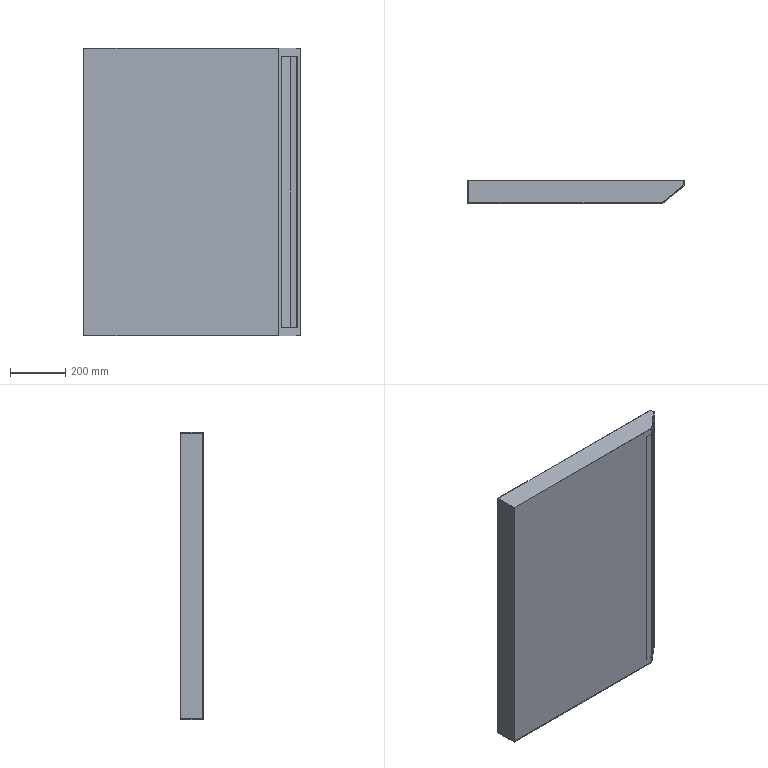Part | SolidWorks | features ICE 6, Extrusion 1, Shell 1 | 4 solids | 46 faces | box 782 x 83 x 1038 mm | volume 2557655 mm3 | plane 46
STEP:
#1=CARTESIAN_POINT('',(2.,2.,2.));
#2=VERTEX_POINT('',#1);
#3=CARTESIAN_POINT('',(703.425,2.,2.));
#4=VERTEX_POINT('',#3);
#5=CARTESIAN_POINT('',(0.,2.,2.));
#6=DIRECTION('',(1.,0.,0.));
#7=VECTOR('',#6,1000.);
#8=LINE('',#5,#7);
#9=EDGE_CURVE('',#2,#4,#8,.T.);
#10=ORIENTED_EDGE('',*,*,#9,.F.);
#11=CARTESIAN_POINT('',(2.,2.,1036.));
#12=VERTEX_POINT('',#11);
#13=CARTESIAN_POINT('',(2.,2.,1038.));
#14=DIRECTION('',(0.,0.,-1.));
#15=VECTOR('',#14,1000.);
#16=LINE('',#13,#15);
#17=EDGE_CURVE('',#12,#2,#16,.T.);
#18=ORIENTED_EDGE('',*,*,#17,.F.);
#19=CARTESIAN_POINT('',(703.425,2.,1036.));
#20=VERTEX_POINT('',#19);
#21=CARTESIAN_POINT('',(0.,2.,1036.));
#22=DIRECTION('',(1.,0.,0.));
#23=VECTOR('',#22,1000.);
#24=LINE('',#21,#23);
#25=EDGE_CURVE('',#12,#20,#24,.T.);
#26=ORIENTED_EDGE('',*,*,#25,.T.);
#27=CARTESIAN_POINT('',(703.425,2.,1038.));
#28=DIRECTION('',(0.,0.,-1.));
#29=VECTOR('',#28,1000.);
#30=LINE('',#27,#29);
#31=EDGE_CURVE('',#20,#4,#30,.T.);
#32=ORIENTED_EDGE('',*,*,#31,.T.);
#33=EDGE_LOOP('',(#10,#18,#26,#32));
#34=FACE_OUTER_BOUND('',#33,.T.);
#35=CARTESIAN_POINT('',(677.425,2.,1012.));
#36=VERTEX_POINT('',#35);
#37=CARTESIAN_POINT('',(679.425,2.,1012.));
#38=VERTEX_POINT('',#37);
#39=CARTESIAN_POINT('',(677.425,2.,1012.));
#40=DIRECTION('',(1.,0.,0.));
#41=VECTOR('',#40,1000.);
#42=LINE('',#39,#41);
#43=EDGE_CURVE('',#36,#38,#42,.T.);
#44=ORIENTED_EDGE('',*,*,#43,.F.);
#45=CARTESIAN_POINT('',(677.425,2.,26.));
#46=VERTEX_POINT('',#45);
#47=CARTESIAN_POINT('',(677.425,2.,26.));
#48=DIRECTION('',(0.,0.,1.));
#49=VECTOR('',#48,1000.);
#50=LINE('',#47,#49);
#51=EDGE_CURVE('',#46,#36,#50,.T.);
#52=ORIENTED_EDGE('',*,*,#51,.F.);
#53=CARTESIAN_POINT('',(679.425,2.,26.));
#54=VERTEX_POINT('',#53);
#55=CARTESIAN_POINT('',(677.425,2.,26.));
#56=DIRECTION('',(-1.,0.,0.));
#57=VECTOR('',#56,1000.);
#58=LINE('',#55,#57);
#59=EDGE_CURVE('',#54,#46,#58,.T.);
#60=ORIENTED_EDGE('',*,*,#59,.F.);
#61=CARTESIAN_POINT('',(679.425,2.,26.));
#62=DIRECTION('',(0.,0.,-1.));
#63=VECTOR('',#62,1000.);
#64=LINE('',#61,#63);
#65=EDGE_CURVE('',#38,#54,#64,.T.);
#66=ORIENTED_EDGE('',*,*,#65,.F.);
#67=EDGE_LOOP('',(#44,#52,#60,#66));
#68=FACE_BOUND('',#67,.T.);
#69=CARTESIAN_POINT('',(704.153,2.,1038.));
#70=DIRECTION('',(0.,1.,0.));
#71=DIRECTION('',(-1.,0.,0.));
#72=AXIS2_PLACEMENT_3D('',#69,#70,#71);
#73=PLANE('',#72);
#74=ADVANCED_FACE('',(#34,#68),#73,.T.);
#75=CARTESIAN_POINT('',(0.,0.,0.));
#76=VERTEX_POINT('',#75);
#77=CARTESIAN_POINT('',(704.153,0.,0.));
#78=VERTEX_POINT('',#77);
#79=CARTESIAN_POINT('',(704.153,0.,0.));
#80=DIRECTION('',(1.,0.,0.));
#81=VECTOR('',#80,1000.);
#82=LINE('',#79,#81);
#83=EDGE_CURVE('',#76,#78,#82,.T.);
#84=ORIENTED_EDGE('',*,*,#83,.T.);
#85=CARTESIAN_POINT('',(704.153,0.,1038.));
#86=VERTEX_POINT('',#85);
#87=CARTESIAN_POINT('',(704.153,0.,1038.));
#88=DIRECTION('',(0.,0.,-1.));
#89=VECTOR('',#88,1000.);
#90=LINE('',#87,#89);
#91=EDGE_CURVE('',#86,#78,#90,.T.);
#92=ORIENTED_EDGE('',*,*,#91,.F.);
#93=CARTESIAN_POINT('',(0.,0.,1038.));
#94=VERTEX_POINT('',#93);
#95=CARTESIAN_POINT('',(704.153,0.,1038.));
#96=DIRECTION('',(1.,0.,0.));
#97=VECTOR('',#96,1000.);
#98=LINE('',#95,#97);
#99=EDGE_CURVE('',#94,#86,#98,.T.);
#100=ORIENTED_EDGE('',*,*,#99,.F.);
#101=CARTESIAN_POINT('',(0.,0.,1038.));
#102=DIRECTION('',(0.,0.,-1.));
#103=VECTOR('',#102,1000.);
#104=LINE('',#101,#103);
#105=EDGE_CURVE('',#94,#76,#104,.T.);
#106=ORIENTED_EDGE('',*,*,#105,.T.);
#107=EDGE_LOOP('',(#84,#92,#100,#106));
#108=FACE_OUTER_BOUND('',#107,.T.);
#109=CARTESIAN_POINT('',(704.153,0.,1038.));
#110=DIRECTION('',(0.,1.,0.));
#111=DIRECTION('',(-1.,0.,0.));
#112=AXIS2_PLACEMENT_3D('',#109,#110,#111);
#113=PLANE('',#112);
#114=ADVANCED_FACE('',(#108),#113,.F.);
#115=CARTESIAN_POINT('',(714.35,8.556,28.));
#116=VERTEX_POINT('',#115);
#117=CARTESIAN_POINT('',(771.803,56.765,28.));
#118=VERTEX_POINT('',#117);
#119=CARTESIAN_POINT('',(714.35,8.556,28.));
#120=DIRECTION('',(0.766,0.6428,0.));
#121=VECTOR('',#120,1000.);
#122=LINE('',#119,#121);
#123=EDGE_CURVE('',#116,#118,#122,.T.);
#124=ORIENTED_EDGE('',*,*,#123,.F.);
#125=CARTESIAN_POINT('',(714.35,8.556,1010.));
#126=VERTEX_POINT('',#125);
#127=CARTESIAN_POINT('',(714.35,8.556,1010.));
#128=DIRECTION('',(0.,0.,-1.));
#129=VECTOR('',#128,1000.);
#130=LINE('',#127,#129);
#131=EDGE_CURVE('',#126,#116,#130,.T.);
#132=ORIENTED_EDGE('',*,*,#131,.F.);
#133=CARTESIAN_POINT('',(771.803,56.765,1010.));
#134=VERTEX_POINT('',#133);
#135=CARTESIAN_POINT('',(714.35,8.556,1010.));
#136=DIRECTION('',(-0.766,-0.6428,0.));
#137=VECTOR('',#136,1000.);
#138=LINE('',#135,#137);
#139=EDGE_CURVE('',#134,#126,#138,.T.);
#140=ORIENTED_EDGE('',*,*,#139,.F.);
#141=CARTESIAN_POINT('',(771.803,56.765,1010.));
#142=DIRECTION('',(0.,0.,1.));
#143=VECTOR('',#142,1000.);
#144=LINE('',#141,#143);
#145=EDGE_CURVE('',#118,#134,#144,.T.);
#146=ORIENTED_EDGE('',*,*,#145,.F.);
#147=EDGE_LOOP('',(#124,#132,#140,#146));
#148=FACE_BOUND('',#147,.T.);
#149=CARTESIAN_POINT('',(782.,65.322,0.));
#150=VERTEX_POINT('',#149);
#151=CARTESIAN_POINT('',(784.,67.,0.));
#152=DIRECTION('',(0.766,0.6428,0.));
#153=VECTOR('',#152,1000.);
#154=LINE('',#151,#153);
#155=EDGE_CURVE('',#78,#150,#154,.T.);
#156=ORIENTED_EDGE('',*,*,#155,.T.);
#157=CARTESIAN_POINT('',(782.,65.322,1038.));
#158=VERTEX_POINT('',#157);
#159=CARTESIAN_POINT('',(782.,65.322,1038.));
#160=DIRECTION('',(0.,0.,1.));
#161=VECTOR('',#160,1000.);
#162=LINE('',#159,#161);
#163=EDGE_CURVE('',#150,#158,#162,.T.);
#164=ORIENTED_EDGE('',*,*,#163,.T.);
#165=CARTESIAN_POINT('',(784.,67.,1038.));
#166=DIRECTION('',(0.766,0.6428,0.));
#167=VECTOR('',#166,1000.);
#168=LINE('',#165,#167);
#169=EDGE_CURVE('',#86,#158,#168,.T.);
#170=ORIENTED_EDGE('',*,*,#169,.F.);
#171=ORIENTED_EDGE('',*,*,#91,.T.);
#172=EDGE_LOOP('',(#156,#164,#170,#171));
#173=FACE_OUTER_BOUND('',#172,.T.);
#174=CARTESIAN_POINT('',(784.,67.,1038.));
#175=DIRECTION('',(-0.6428,0.766,0.));
#176=DIRECTION('',(-0.766,-0.6428,0.));
#177=AXIS2_PLACEMENT_3D('',#174,#175,#176);
#178=PLANE('',#177);
#179=ADVANCED_FACE('',(#148,#173),#178,.F.);
#180=CARTESIAN_POINT('',(780.,83.,1036.));
#181=VERTEX_POINT('',#180);
#182=CARTESIAN_POINT('',(780.,83.,2.));
#183=VERTEX_POINT('',#182);
#184=CARTESIAN_POINT('',(780.,83.,1038.));
#185=DIRECTION('',(0.,0.,-1.));
#186=VECTOR('',#185,1000.);
#187=LINE('',#184,#186);
#188=EDGE_CURVE('',#181,#183,#187,.T.);
#189=ORIENTED_EDGE('',*,*,#188,.F.);
#190=CARTESIAN_POINT('',(2.,83.,1036.));
#191=VERTEX_POINT('',#190);
#192=CARTESIAN_POINT('',(0.,83.,1036.));
#193=DIRECTION('',(-1.,0.,0.));
#194=VECTOR('',#193,1000.);
#195=LINE('',#192,#194);
#196=EDGE_CURVE('',#181,#191,#195,.T.);
#197=ORIENTED_EDGE('',*,*,#196,.T.);
#198=CARTESIAN_POINT('',(2.,83.,2.));
#199=VERTEX_POINT('',#198);
#200=CARTESIAN_POINT('',(2.,83.,1038.));
#201=DIRECTION('',(0.,0.,-1.));
#202=VECTOR('',#201,1000.);
#203=LINE('',#200,#202);
#204=EDGE_CURVE('',#191,#199,#203,.T.);
#205=ORIENTED_EDGE('',*,*,#204,.T.);
#206=CARTESIAN_POINT('',(0.,83.,2.));
#207=DIRECTION('',(-1.,0.,0.));
#208=VECTOR('',#207,1000.);
#209=LINE('',#206,#208);
#210=EDGE_CURVE('',#183,#199,#209,.T.);
#211=ORIENTED_EDGE('',*,*,#210,.F.);
#212=EDGE_LOOP('',(#189,#197,#205,#211));
#213=FACE_BOUND('',#212,.T.);
#214=CARTESIAN_POINT('',(782.,83.,1038.));
#215=VERTEX_POINT('',#214);
#216=CARTESIAN_POINT('',(0.,83.,1038.));
#217=VERTEX_POINT('',#216);
#218=CARTESIAN_POINT('',(0.,83.,1038.));
#219=DIRECTION('',(-1.,0.,0.));
#220=VECTOR('',#219,1000.);
#221=LINE('',#218,#220);
#222=EDGE_CURVE('',#215,#217,#221,.T.);
#223=ORIENTED_EDGE('',*,*,#222,.F.);
#224=CARTESIAN_POINT('',(782.,83.,0.));
#225=VERTEX_POINT('',#224);
#226=CARTESIAN_POINT('',(782.,83.,1038.));
#227=DIRECTION('',(0.,0.,-1.));
#228=VECTOR('',#227,1000.);
#229=LINE('',#226,#228);
#230=EDGE_CURVE('',#215,#225,#229,.T.);
#231=ORIENTED_EDGE('',*,*,#230,.T.);
#232=CARTESIAN_POINT('',(0.,83.,0.));
#233=VERTEX_POINT('',#232);
#234=CARTESIAN_POINT('',(0.,83.,0.));
#235=DIRECTION('',(-1.,0.,0.));
#236=VECTOR('',#235,1000.);
#237=LINE('',#234,#236);
#238=EDGE_CURVE('',#225,#233,#237,.T.);
#239=ORIENTED_EDGE('',*,*,#238,.T.);
#240=CARTESIAN_POINT('',(0.,83.,1038.));
#241=DIRECTION('',(0.,0.,-1.));
#242=VECTOR('',#241,1000.);
#243=LINE('',#240,#242);
#244=EDGE_CURVE('',#217,#233,#243,.T.);
#245=ORIENTED_EDGE('',*,*,#244,.F.);
#246=EDGE_LOOP('',(#223,#231,#239,#245));
#247=FACE_OUTER_BOUND('',#246,.T.);
#248=CARTESIAN_POINT('',(0.,83.,1038.));
#249=DIRECTION('',(0.,-1.,0.));
#250=DIRECTION('',(0.,0.,-1.));
#251=AXIS2_PLACEMENT_3D('',#248,#249,#250);
#252=PLANE('',#251);
#253=ADVANCED_FACE('',(#213,#247),#252,.F.);
#254=CARTESIAN_POINT('',(0.,0.,0.));
#255=DIRECTION('',(0.,-1.,0.));
#256=VECTOR('',#255,1000.);
#257=LINE('',#254,#256);
#258=EDGE_CURVE('',#233,#76,#257,.T.);
#259=ORIENTED_EDGE('',*,*,#258,.T.);
#260=ORIENTED_EDGE('',*,*,#105,.F.);
#261=CARTESIAN_POINT('',(0.,0.,1038.));
#262=DIRECTION('',(0.,-1.,0.));
#263=VECTOR('',#262,1000.);
#264=LINE('',#261,#263);
#265=EDGE_CURVE('',#217,#94,#264,.T.);
#266=ORIENTED_EDGE('',*,*,#265,.F.);
#267=ORIENTED_EDGE('',*,*,#244,.T.);
#268=EDGE_LOOP('',(#259,#260,#266,#267));
#269=FACE_OUTER_BOUND('',#268,.T.);
#270=CARTESIAN_POINT('',(0.,0.,1038.));
#271=DIRECTION('',(1.,0.,0.));
#272=DIRECTION('',(0.,0.,-1.));
#273=AXIS2_PLACEMENT_3D('',#270,#271,#272);
#274=PLANE('',#273);
#275=ADVANCED_FACE('',(#269),#274,.F.);
#276=ORIENTED_EDGE('',*,*,#169,.T.);
#277=CARTESIAN_POINT('',(782.,134.153,1038.));
#278=DIRECTION('',(0.,-1.,0.));
#279=VECTOR('',#278,1000.);
#280=LINE('',#277,#279);
#281=EDGE_CURVE('',#215,#158,#280,.T.);
#282=ORIENTED_EDGE('',*,*,#281,.F.);
#283=ORIENTED_EDGE('',*,*,#222,.T.);
#284=ORIENTED_EDGE('',*,*,#265,.T.);
#285=ORIENTED_EDGE('',*,*,#99,.T.);
#286=EDGE_LOOP('',(#276,#282,#283,#284,#285));
#287=FACE_OUTER_BOUND('',#286,.T.);
#288=CARTESIAN_POINT('',(0.,0.,1038.));
#289=DIRECTION('',(0.,0.,-1.));
#290=DIRECTION('',(-1.,0.,0.));
#291=AXIS2_PLACEMENT_3D('',#288,#289,#290);
#292=PLANE('',#291);
#293=ADVANCED_FACE('',(#287),#292,.F.);
#294=CARTESIAN_POINT('',(782.,0.,0.));
#295=DIRECTION('',(0.,1.,0.));
#296=VECTOR('',#295,1000.);
#297=LINE('',#294,#296);
#298=EDGE_CURVE('',#150,#225,#297,.T.);
#299=ORIENTED_EDGE('',*,*,#298,.F.);
#300=ORIENTED_EDGE('',*,*,#155,.F.);
#301=ORIENTED_EDGE('',*,*,#83,.F.);
#302=ORIENTED_EDGE('',*,*,#258,.F.);
#303=ORIENTED_EDGE('',*,*,#238,.F.);
#304=EDGE_LOOP('',(#299,#300,#301,#302,#303));
#305=FACE_OUTER_BOUND('',#304,.T.);
#306=CARTESIAN_POINT('',(0.,0.,0.));
#307=DIRECTION('',(0.,0.,-1.));
#308=DIRECTION('',(-1.,0.,0.));
#309=AXIS2_PLACEMENT_3D('',#306,#307,#308);
#310=PLANE('',#309);
#311=ADVANCED_FACE('',(#305),#310,.T.);
#312=ORIENTED_EDGE('',*,*,#298,.T.);
#313=ORIENTED_EDGE('',*,*,#230,.F.);
#314=ORIENTED_EDGE('',*,*,#281,.T.);
#315=ORIENTED_EDGE('',*,*,#163,.F.);
#316=EDGE_LOOP('',(#312,#313,#314,#315));
#317=FACE_OUTER_BOUND('',#316,.T.);
#318=CARTESIAN_POINT('',(782.,134.153,-153.));
#319=DIRECTION('',(-1.,0.,0.));
#320=DIRECTION('',(0.,0.,1.));
#321=AXIS2_PLACEMENT_3D('',#318,#319,#320);
#322=PLANE('',#321);
#323=ADVANCED_FACE('',(#317),#322,.F.);
#324=CARTESIAN_POINT('',(713.064,10.088,28.));
#325=VERTEX_POINT('',#324);
#326=CARTESIAN_POINT('',(713.064,10.088,1010.));
#327=VERTEX_POINT('',#326);
#328=CARTESIAN_POINT('',(713.064,10.088,1038.));
#329=DIRECTION('',(0.,0.,1.));
#330=VECTOR('',#329,1000.);
#331=LINE('',#328,#330);
#332=EDGE_CURVE('',#325,#327,#331,.T.);
#333=ORIENTED_EDGE('',*,*,#332,.F.);
#334=CARTESIAN_POINT('',(770.517,58.298,28.));
#335=VERTEX_POINT('',#334);
#336=CARTESIAN_POINT('',(782.714,68.532,28.));
#337=DIRECTION('',(-0.766,-0.6428,0.));
#338=VECTOR('',#337,1000.);
#339=LINE('',#336,#338);
#340=EDGE_CURVE('',#335,#325,#339,.T.);
#341=ORIENTED_EDGE('',*,*,#340,.F.);
#342=CARTESIAN_POINT('',(770.517,58.298,1010.));
#343=VERTEX_POINT('',#342);
#344=CARTESIAN_POINT('',(770.517,58.298,1038.));
#345=DIRECTION('',(0.,0.,-1.));
#346=VECTOR('',#345,1000.);
#347=LINE('',#344,#346);
#348=EDGE_CURVE('',#343,#335,#347,.T.);
#349=ORIENTED_EDGE('',*,*,#348,.F.);
#350=CARTESIAN_POINT('',(782.714,68.532,1010.));
#351=DIRECTION('',(0.766,0.6428,0.));
#352=VECTOR('',#351,1000.);
#353=LINE('',#350,#352);
#354=EDGE_CURVE('',#327,#343,#353,.T.);
#355=ORIENTED_EDGE('',*,*,#354,.F.);
#356=EDGE_LOOP('',(#333,#341,#349,#355));
#357=FACE_BOUND('',#356,.T.);
#358=CARTESIAN_POINT('',(780.,66.254,2.));
#359=VERTEX_POINT('',#358);
#360=CARTESIAN_POINT('',(289.653,-345.195,2.));
#361=DIRECTION('',(0.766,0.6428,0.));
#362=VECTOR('',#361,1000.);
#363=LINE('',#360,#362);
#364=EDGE_CURVE('',#4,#359,#363,.T.);
#365=ORIENTED_EDGE('',*,*,#364,.F.);
#366=ORIENTED_EDGE('',*,*,#31,.F.);
#367=CARTESIAN_POINT('',(780.,66.254,1036.));
#368=VERTEX_POINT('',#367);
#369=CARTESIAN_POINT('',(289.653,-345.195,1036.));
#370=DIRECTION('',(0.766,0.6428,0.));
#371=VECTOR('',#370,1000.);
#372=LINE('',#369,#371);
#373=EDGE_CURVE('',#20,#368,#372,.T.);
#374=ORIENTED_EDGE('',*,*,#373,.T.);
#375=CARTESIAN_POINT('',(780.,66.254,1038.));
#376=DIRECTION('',(0.,0.,1.));
#377=VECTOR('',#376,1000.);
#378=LINE('',#375,#377);
#379=EDGE_CURVE('',#359,#368,#378,.T.);
#380=ORIENTED_EDGE('',*,*,#379,.F.);
#381=EDGE_LOOP('',(#365,#366,#374,#380));
#382=FACE_OUTER_BOUND('',#381,.T.);
#383=CARTESIAN_POINT('',(782.714,68.532,1038.));
#384=DIRECTION('',(-0.6428,0.766,0.));
#385=DIRECTION('',(-0.766,-0.6428,0.));
#386=AXIS2_PLACEMENT_3D('',#383,#384,#385);
#387=PLANE('',#386);
#388=ADVANCED_FACE('',(#357,#382),#387,.T.);
#389=CARTESIAN_POINT('',(2.,0.,2.));
#390=DIRECTION('',(0.,-1.,0.));
#391=VECTOR('',#390,1000.);
#392=LINE('',#389,#391);
#393=EDGE_CURVE('',#199,#2,#392,.T.);
#394=ORIENTED_EDGE('',*,*,#393,.F.);
#395=ORIENTED_EDGE('',*,*,#204,.F.);
#396=CARTESIAN_POINT('',(2.,0.,1036.));
#397=DIRECTION('',(0.,-1.,0.));
#398=VECTOR('',#397,1000.);
#399=LINE('',#396,#398);
#400=EDGE_CURVE('',#191,#12,#399,.T.);
#401=ORIENTED_EDGE('',*,*,#400,.T.);
#402=ORIENTED_EDGE('',*,*,#17,.T.);
#403=EDGE_LOOP('',(#394,#395,#401,#402));
#404=FACE_OUTER_BOUND('',#403,.T.);
#405=CARTESIAN_POINT('',(2.,0.,1038.));
#406=DIRECTION('',(1.,0.,0.));
#407=DIRECTION('',(0.,0.,-1.));
#408=AXIS2_PLACEMENT_3D('',#405,#406,#407);
#409=PLANE('',#408);
#410=ADVANCED_FACE('',(#404),#409,.T.);
#411=ORIENTED_EDGE('',*,*,#373,.F.);
#412=ORIENTED_EDGE('',*,*,#25,.F.);
#413=ORIENTED_EDGE('',*,*,#400,.F.);
#414=ORIENTED_EDGE('',*,*,#196,.F.);
#415=CARTESIAN_POINT('',(780.,134.153,1036.));
#416=DIRECTION('',(0.,-1.,0.));
#417=VECTOR('',#416,1000.);
#418=LINE('',#415,#417);
#419=EDGE_CURVE('',#181,#368,#418,.T.);
#420=ORIENTED_EDGE('',*,*,#419,.T.);
#421=EDGE_LOOP('',(#411,#412,#413,#414,#420));
#422=FACE_OUTER_BOUND('',#421,.T.);
#423=CARTESIAN_POINT('',(0.,0.,1036.));
#424=DIRECTION('',(0.,0.,-1.));
#425=DIRECTION('',(-1.,0.,0.));
#426=AXIS2_PLACEMENT_3D('',#423,#424,#425);
#427=PLANE('',#426);
#428=ADVANCED_FACE('',(#422),#427,.T.);
#429=CARTESIAN_POINT('',(780.,0.,2.));
#430=DIRECTION('',(0.,1.,0.));
#431=VECTOR('',#430,1000.);
#432=LINE('',#429,#431);
#433=EDGE_CURVE('',#359,#183,#432,.T.);
#434=ORIENTED_EDGE('',*,*,#433,.T.);
#435=ORIENTED_EDGE('',*,*,#210,.T.);
#436=ORIENTED_EDGE('',*,*,#393,.T.);
#437=ORIENTED_EDGE('',*,*,#9,.T.);
#438=ORIENTED_EDGE('',*,*,#364,.T.);
#439=EDGE_LOOP('',(#434,#435,#436,#437,#438));
#440=FACE_OUTER_BOUND('',#439,.T.);
#441=CARTESIAN_POINT('',(0.,0.,2.));
#442=DIRECTION('',(0.,0.,-1.));
#443=DIRECTION('',(-1.,0.,0.));
#444=AXIS2_PLACEMENT_3D('',#441,#442,#443);
#445=PLANE('',#444);
#446=ADVANCED_FACE('',(#440),#445,.F.);
#447=ORIENTED_EDGE('',*,*,#433,.F.);
#448=ORIENTED_EDGE('',*,*,#379,.T.);
#449=ORIENTED_EDGE('',*,*,#419,.F.);
#450=ORIENTED_EDGE('',*,*,#188,.T.);
#451=EDGE_LOOP('',(#447,#448,#449,#450));
#452=FACE_OUTER_BOUND('',#451,.T.);
#453=CARTESIAN_POINT('',(780.,134.153,-153.));
#454=DIRECTION('',(-1.,0.,0.));
#455=DIRECTION('',(0.,0.,1.));
#456=AXIS2_PLACEMENT_3D('',#453,#454,#455);
#457=PLANE('',#456);
#458=ADVANCED_FACE('',(#452),#457,.T.);
#459=ORIENTED_EDGE('',*,*,#332,.T.);
#460=CARTESIAN_POINT('',(293.966,509.549,1010.));
#461=DIRECTION('',(0.6428,-0.766,0.));
#462=VECTOR('',#461,1000.);
#463=LINE('',#460,#462);
#464=EDGE_CURVE('',#327,#126,#463,.T.);
#465=ORIENTED_EDGE('',*,*,#464,.T.);
#466=ORIENTED_EDGE('',*,*,#131,.T.);
#467=CARTESIAN_POINT('',(293.966,509.549,28.));
#468=DIRECTION('',(0.6428,-0.766,0.));
#469=VECTOR('',#468,1000.);
#470=LINE('',#467,#469);
#471=EDGE_CURVE('',#325,#116,#470,.T.);
#472=ORIENTED_EDGE('',*,*,#471,.F.);
#473=EDGE_LOOP('',(#459,#465,#466,#472));
#474=FACE_OUTER_BOUND('',#473,.T.);
#475=CARTESIAN_POINT('',(293.966,509.549,1010.));
#476=DIRECTION('',(-0.766,-0.6428,0.));
#477=DIRECTION('',(0.6428,-0.766,0.));
#478=AXIS2_PLACEMENT_3D('',#475,#476,#477);
#479=PLANE('',#478);
#480=ADVANCED_FACE('',(#474),#479,.F.);
#481=ORIENTED_EDGE('',*,*,#354,.T.);
#482=CARTESIAN_POINT('',(351.42,557.759,1010.));
#483=DIRECTION('',(0.6428,-0.766,0.));
#484=VECTOR('',#483,1000.);
#485=LINE('',#482,#484);
#486=EDGE_CURVE('',#343,#134,#485,.T.);
#487=ORIENTED_EDGE('',*,*,#486,.T.);
#488=ORIENTED_EDGE('',*,*,#139,.T.);
#489=ORIENTED_EDGE('',*,*,#464,.F.);
#490=EDGE_LOOP('',(#481,#487,#488,#489));
#491=FACE_OUTER_BOUND('',#490,.T.);
#492=CARTESIAN_POINT('',(293.966,509.549,1010.));
#493=DIRECTION('',(0.,0.,1.));
#494=DIRECTION('',(1.,0.,0.));
#495=AXIS2_PLACEMENT_3D('',#492,#493,#494);
#496=PLANE('',#495);
#497=ADVANCED_FACE('',(#491),#496,.F.);
#498=ORIENTED_EDGE('',*,*,#348,.T.);
#499=CARTESIAN_POINT('',(351.42,557.759,28.));
#500=DIRECTION('',(0.6428,-0.766,0.));
#501=VECTOR('',#500,1000.);
#502=LINE('',#499,#501);
#503=EDGE_CURVE('',#335,#118,#502,.T.);
#504=ORIENTED_EDGE('',*,*,#503,.T.);
#505=ORIENTED_EDGE('',*,*,#145,.T.);
#506=ORIENTED_EDGE('',*,*,#486,.F.);
#507=EDGE_LOOP('',(#498,#504,#505,#506));
#508=FACE_OUTER_BOUND('',#507,.T.);
#509=CARTESIAN_POINT('',(351.42,557.759,1010.));
#510=DIRECTION('',(0.766,0.6428,0.));
#511=DIRECTION('',(-0.6428,0.766,0.));
#512=AXIS2_PLACEMENT_3D('',#509,#510,#511);
#513=PLANE('',#512);
#514=ADVANCED_FACE('',(#508),#513,.F.);
#515=ORIENTED_EDGE('',*,*,#340,.T.);
#516=ORIENTED_EDGE('',*,*,#471,.T.);
#517=ORIENTED_EDGE('',*,*,#123,.T.);
#518=ORIENTED_EDGE('',*,*,#503,.F.);
#519=EDGE_LOOP('',(#515,#516,#517,#518));
#520=FACE_OUTER_BOUND('',#519,.T.);
#521=CARTESIAN_POINT('',(293.966,509.549,28.));
#522=DIRECTION('',(0.,0.,-1.));
#523=DIRECTION('',(-1.,0.,0.));
#524=AXIS2_PLACEMENT_3D('',#521,#522,#523);
#525=PLANE('',#524);
#526=ADVANCED_FACE('',(#520),#525,.F.);
#527=ORIENTED_EDGE('',*,*,#51,.T.);
#528=CARTESIAN_POINT('',(677.425,62.,1012.));
#529=VERTEX_POINT('',#528);
#530=CARTESIAN_POINT('',(677.425,62.,1012.));
#531=DIRECTION('',(0.,-1.,0.));
#532=VECTOR('',#531,1000.);
#533=LINE('',#530,#532);
#534=EDGE_CURVE('',#529,#36,#533,.T.);
#535=ORIENTED_EDGE('',*,*,#534,.F.);
#536=CARTESIAN_POINT('',(677.425,62.,26.));
#537=VERTEX_POINT('',#536);
#538=CARTESIAN_POINT('',(677.425,62.,26.));
#539=DIRECTION('',(0.,0.,1.));
#540=VECTOR('',#539,1000.);
#541=LINE('',#538,#540);
#542=EDGE_CURVE('',#537,#529,#541,.T.);
#543=ORIENTED_EDGE('',*,*,#542,.F.);
#544=CARTESIAN_POINT('',(677.425,62.,26.));
#545=DIRECTION('',(0.,-1.,0.));
#546=VECTOR('',#545,1000.);
#547=LINE('',#544,#546);
#548=EDGE_CURVE('',#537,#46,#547,.T.);
#549=ORIENTED_EDGE('',*,*,#548,.T.);
#550=EDGE_LOOP('',(#527,#535,#543,#549));
#551=FACE_OUTER_BOUND('',#550,.T.);
#552=CARTESIAN_POINT('',(677.425,62.,26.));
#553=DIRECTION('',(1.,0.,0.));
#554=DIRECTION('',(0.,1.,0.));
#555=AXIS2_PLACEMENT_3D('',#552,#553,#554);
#556=PLANE('',#555);
#557=ADVANCED_FACE('',(#551),#556,.F.);
#558=ORIENTED_EDGE('',*,*,#43,.T.);
#559=CARTESIAN_POINT('',(679.425,62.,1012.));
#560=VERTEX_POINT('',#559);
#561=CARTESIAN_POINT('',(679.425,62.,1012.));
#562=DIRECTION('',(0.,-1.,0.));
#563=VECTOR('',#562,1000.);
#564=LINE('',#561,#563);
#565=EDGE_CURVE('',#560,#38,#564,.T.);
#566=ORIENTED_EDGE('',*,*,#565,.F.);
#567=CARTESIAN_POINT('',(677.425,62.,1012.));
#568=DIRECTION('',(1.,0.,0.));
#569=VECTOR('',#568,1000.);
#570=LINE('',#567,#569);
#571=EDGE_CURVE('',#529,#560,#570,.T.);
#572=ORIENTED_EDGE('',*,*,#571,.F.);
#573=ORIENTED_EDGE('',*,*,#534,.T.);
#574=EDGE_LOOP('',(#558,#566,#572,#573));
#575=FACE_OUTER_BOUND('',#574,.T.);
#576=CARTESIAN_POINT('',(677.425,62.,1012.));
#577=DIRECTION('',(0.,0.,-1.));
#578=DIRECTION('',(-1.,0.,0.));
#579=AXIS2_PLACEMENT_3D('',#576,#577,#578);
#580=PLANE('',#579);
#581=ADVANCED_FACE('',(#575),#580,.F.);
#582=ORIENTED_EDGE('',*,*,#65,.T.);
#583=CARTESIAN_POINT('',(679.425,62.,26.));
#584=VERTEX_POINT('',#583);
#585=CARTESIAN_POINT('',(679.425,62.,26.));
#586=DIRECTION('',(0.,-1.,0.));
#587=VECTOR('',#586,1000.);
#588=LINE('',#585,#587);
#589=EDGE_CURVE('',#584,#54,#588,.T.);
#590=ORIENTED_EDGE('',*,*,#589,.F.);
#591=CARTESIAN_POINT('',(679.425,62.,26.));
#592=DIRECTION('',(0.,0.,-1.));
#593=VECTOR('',#592,1000.);
#594=LINE('',#591,#593);
#595=EDGE_CURVE('',#560,#584,#594,.T.);
#596=ORIENTED_EDGE('',*,*,#595,.F.);
#597=ORIENTED_EDGE('',*,*,#565,.T.);
#598=EDGE_LOOP('',(#582,#590,#596,#597));
#599=FACE_OUTER_BOUND('',#598,.T.);
#600=CARTESIAN_POINT('',(679.425,62.,26.));
#601=DIRECTION('',(-1.,0.,0.));
#602=DIRECTION('',(0.,0.,1.));
#603=AXIS2_PLACEMENT_3D('',#600,#601,#602);
#604=PLANE('',#603);
#605=ADVANCED_FACE('',(#599),#604,.F.);
#606=ORIENTED_EDGE('',*,*,#59,.T.);
#607=ORIENTED_EDGE('',*,*,#548,.F.);
#608=CARTESIAN_POINT('',(677.425,62.,26.));
#609=DIRECTION('',(-1.,0.,0.));
#610=VECTOR('',#609,1000.);
#611=LINE('',#608,#610);
#612=EDGE_CURVE('',#584,#537,#611,.T.);
#613=ORIENTED_EDGE('',*,*,#612,.F.);
#614=ORIENTED_EDGE('',*,*,#589,.T.);
#615=EDGE_LOOP('',(#606,#607,#613,#614));
#616=FACE_OUTER_BOUND('',#615,.T.);
#617=CARTESIAN_POINT('',(677.425,62.,26.));
#618=DIRECTION('',(0.,0.,1.));
#619=DIRECTION('',(1.,0.,0.));
#620=AXIS2_PLACEMENT_3D('',#617,#618,#619);
#621=PLANE('',#620);
#622=ADVANCED_FACE('',(#616),#621,.F.);
#623=ORIENTED_EDGE('',*,*,#542,.T.);
#624=ORIENTED_EDGE('',*,*,#571,.T.);
#625=ORIENTED_EDGE('',*,*,#595,.T.);
#626=ORIENTED_EDGE('',*,*,#612,.T.);
#627=EDGE_LOOP('',(#623,#624,#625,#626));
#628=FACE_OUTER_BOUND('',#627,.T.);
#629=CARTESIAN_POINT('',(677.425,62.,1012.));
#630=DIRECTION('',(0.,1.,0.));
#631=DIRECTION('',(0.,0.,1.));
#632=AXIS2_PLACEMENT_3D('',#629,#630,#631);
#633=PLANE('',#632);
#634=ADVANCED_FACE('',(#628),#633,.T.);
#635=CLOSED_SHELL('',(#74,#114,#179,#253,#275,#293,#311,#323,#388,#410,#428,#446,#458,#480,#497,#514,#526,#557,#581,#605,#622,#634));
#636=MANIFOLD_SOLID_BREP('',#635);
#637=CARTESIAN_POINT('',(679.425,2.,26.));
#638=VERTEX_POINT('',#637);
#639=CARTESIAN_POINT('',(679.425,2.,1012.));
#640=VERTEX_POINT('',#639);
#641=CARTESIAN_POINT('',(679.425,2.,26.));
#642=DIRECTION('',(0.,0.,1.));
#643=VECTOR('',#642,1000.);
#644=LINE('',#641,#643);
#645=EDGE_CURVE('',#638,#640,#644,.T.);
#646=ORIENTED_EDGE('',*,*,#645,.T.);
#647=CARTESIAN_POINT('',(679.425,62.,1012.));
#648=VERTEX_POINT('',#647);
#649=CARTESIAN_POINT('',(679.425,62.,1012.));
#650=DIRECTION('',(0.,-1.,0.));
#651=VECTOR('',#650,1000.);
#652=LINE('',#649,#651);
#653=EDGE_CURVE('',#648,#640,#652,.T.);
#654=ORIENTED_EDGE('',*,*,#653,.F.);
#655=CARTESIAN_POINT('',(679.425,62.,26.));
#656=VERTEX_POINT('',#655);
#657=CARTESIAN_POINT('',(679.425,62.,26.));
#658=DIRECTION('',(0.,0.,1.));
#659=VECTOR('',#658,1000.);
#660=LINE('',#657,#659);
#661=EDGE_CURVE('',#656,#648,#660,.T.);
#662=ORIENTED_EDGE('',*,*,#661,.F.);
#663=CARTESIAN_POINT('',(679.425,62.,26.));
#664=DIRECTION('',(0.,-1.,0.));
#665=VECTOR('',#664,1000.);
#666=LINE('',#663,#665);
#667=EDGE_CURVE('',#656,#638,#666,.T.);
#668=ORIENTED_EDGE('',*,*,#667,.T.);
#669=EDGE_LOOP('',(#646,#654,#662,#668));
#670=FACE_OUTER_BOUND('',#669,.T.);
#671=CARTESIAN_POINT('',(679.425,62.,26.));
#672=DIRECTION('',(-1.,0.,0.));
#673=DIRECTION('',(0.,0.,1.));
#674=AXIS2_PLACEMENT_3D('',#671,#672,#673);
#675=PLANE('',#674);
#676=ADVANCED_FACE('',(#670),#675,.T.);
#677=ORIENTED_EDGE('',*,*,#661,.T.);
#678=CARTESIAN_POINT('',(774.93,62.,1012.));
#679=VERTEX_POINT('',#678);
#680=CARTESIAN_POINT('',(679.425,62.,1012.));
#681=DIRECTION('',(-1.,0.,0.));
#682=VECTOR('',#681,1000.);
#683=LINE('',#680,#682);
#684=EDGE_CURVE('',#679,#648,#683,.T.);
#685=ORIENTED_EDGE('',*,*,#684,.F.);
#686=CARTESIAN_POINT('',(774.93,62.,26.));
#687=VERTEX_POINT('',#686);
#688=CARTESIAN_POINT('',(774.93,62.,26.));
#689=DIRECTION('',(0.,0.,1.));
#690=VECTOR('',#689,1000.);
#691=LINE('',#688,#690);
#692=EDGE_CURVE('',#687,#679,#691,.T.);
#693=ORIENTED_EDGE('',*,*,#692,.F.);
#694=CARTESIAN_POINT('',(679.425,62.,26.));
#695=DIRECTION('',(-1.,0.,0.));
#696=VECTOR('',#695,1000.);
#697=LINE('',#694,#696);
#698=EDGE_CURVE('',#687,#656,#697,.T.);
#699=ORIENTED_EDGE('',*,*,#698,.T.);
#700=EDGE_LOOP('',(#677,#685,#693,#699));
#701=FACE_OUTER_BOUND('',#700,.T.);
#702=CARTESIAN_POINT('',(679.425,62.,26.));
#703=DIRECTION('',(0.,1.,0.));
#704=DIRECTION('',(-1.,0.,0.));
#705=AXIS2_PLACEMENT_3D('',#702,#703,#704);
#706=PLANE('',#705);
#707=ADVANCED_FACE('',(#701),#706,.T.);
#708=ORIENTED_EDGE('',*,*,#692,.T.);
#709=CARTESIAN_POINT('',(772.546,60.,1012.));
#710=VERTEX_POINT('',#709);
#711=CARTESIAN_POINT('',(774.93,62.,1012.));
#712=DIRECTION('',(0.766,0.6428,0.));
#713=VECTOR('',#712,1000.);
#714=LINE('',#711,#713);
#715=EDGE_CURVE('',#710,#679,#714,.T.);
#716=ORIENTED_EDGE('',*,*,#715,.F.);
#717=CARTESIAN_POINT('',(772.546,60.,26.));
#718=VERTEX_POINT('',#717);
#719=CARTESIAN_POINT('',(772.546,60.,26.));
#720=DIRECTION('',(0.,0.,1.));
#721=VECTOR('',#720,1000.);
#722=LINE('',#719,#721);
#723=EDGE_CURVE('',#718,#710,#722,.T.);
#724=ORIENTED_EDGE('',*,*,#723,.F.);
#725=CARTESIAN_POINT('',(774.93,62.,26.));
#726=DIRECTION('',(0.766,0.6428,0.));
#727=VECTOR('',#726,1000.);
#728=LINE('',#725,#727);
#729=EDGE_CURVE('',#718,#687,#728,.T.);
#730=ORIENTED_EDGE('',*,*,#729,.T.);
#731=EDGE_LOOP('',(#708,#716,#724,#730));
#732=FACE_OUTER_BOUND('',#731,.T.);
#733=CARTESIAN_POINT('',(774.93,62.,26.));
#734=DIRECTION('',(0.6428,-0.766,0.));
#735=DIRECTION('',(0.766,0.6428,0.));
#736=AXIS2_PLACEMENT_3D('',#733,#734,#735);
#737=PLANE('',#736);
#738=ADVANCED_FACE('',(#732),#737,.T.);
#739=ORIENTED_EDGE('',*,*,#723,.T.);
#740=CARTESIAN_POINT('',(681.425,60.,1012.));
#741=VERTEX_POINT('',#740);
#742=CARTESIAN_POINT('',(681.425,60.,1012.));
#743=DIRECTION('',(1.,0.,0.));
#744=VECTOR('',#743,1000.);
#745=LINE('',#742,#744);
#746=EDGE_CURVE('',#741,#710,#745,.T.);
#747=ORIENTED_EDGE('',*,*,#746,.F.);
#748=CARTESIAN_POINT('',(681.425,60.,26.));
#749=VERTEX_POINT('',#748);
#750=CARTESIAN_POINT('',(681.425,60.,26.));
#751=DIRECTION('',(0.,0.,1.));
#752=VECTOR('',#751,1000.);
#753=LINE('',#750,#752);
#754=EDGE_CURVE('',#749,#741,#753,.T.);
#755=ORIENTED_EDGE('',*,*,#754,.F.);
#756=CARTESIAN_POINT('',(681.425,60.,26.));
#757=DIRECTION('',(1.,0.,0.));
#758=VECTOR('',#757,1000.);
#759=LINE('',#756,#758);
#760=EDGE_CURVE('',#749,#718,#759,.T.);
#761=ORIENTED_EDGE('',*,*,#760,.T.);
#762=EDGE_LOOP('',(#739,#747,#755,#761));
#763=FACE_OUTER_BOUND('',#762,.T.);
#764=CARTESIAN_POINT('',(681.425,60.,26.));
#765=DIRECTION('',(0.,-1.,0.));
#766=DIRECTION('',(0.,0.,-1.));
#767=AXIS2_PLACEMENT_3D('',#764,#765,#766);
#768=PLANE('',#767);
#769=ADVANCED_FACE('',(#763),#768,.T.);
#770=ORIENTED_EDGE('',*,*,#754,.T.);
#771=CARTESIAN_POINT('',(681.425,4.,1012.));
#772=VERTEX_POINT('',#771);
#773=CARTESIAN_POINT('',(681.425,60.,1012.));
#774=DIRECTION('',(0.,1.,0.));
#775=VECTOR('',#774,1000.);
#776=LINE('',#773,#775);
#777=EDGE_CURVE('',#772,#741,#776,.T.);
#778=ORIENTED_EDGE('',*,*,#777,.F.);
#779=CARTESIAN_POINT('',(681.425,4.,26.));
#780=VERTEX_POINT('',#779);
#781=CARTESIAN_POINT('',(681.425,4.,26.));
#782=DIRECTION('',(0.,0.,1.));
#783=VECTOR('',#782,1000.);
#784=LINE('',#781,#783);
#785=EDGE_CURVE('',#780,#772,#784,.T.);
#786=ORIENTED_EDGE('',*,*,#785,.F.);
#787=CARTESIAN_POINT('',(681.425,60.,26.));
#788=DIRECTION('',(0.,1.,0.));
#789=VECTOR('',#788,1000.);
#790=LINE('',#787,#789);
#791=EDGE_CURVE('',#780,#749,#790,.T.);
#792=ORIENTED_EDGE('',*,*,#791,.T.);
#793=EDGE_LOOP('',(#770,#778,#786,#792));
#794=FACE_OUTER_BOUND('',#793,.T.);
#795=CARTESIAN_POINT('',(681.425,60.,26.));
#796=DIRECTION('',(1.,0.,0.));
#797=DIRECTION('',(0.,0.,-1.));
#798=AXIS2_PLACEMENT_3D('',#795,#796,#797);
#799=PLANE('',#798);
#800=ADVANCED_FACE('',(#794),#799,.T.);
#801=ORIENTED_EDGE('',*,*,#785,.T.);
#802=CARTESIAN_POINT('',(702.697,4.,1012.));
#803=VERTEX_POINT('',#802);
#804=CARTESIAN_POINT('',(681.425,4.,1012.));
#805=DIRECTION('',(-1.,0.,0.));
#806=VECTOR('',#805,1000.);
#807=LINE('',#804,#806);
#808=EDGE_CURVE('',#803,#772,#807,.T.);
#809=ORIENTED_EDGE('',*,*,#808,.F.);
#810=CARTESIAN_POINT('',(702.697,4.,26.));
#811=VERTEX_POINT('',#810);
#812=CARTESIAN_POINT('',(702.697,4.,26.));
#813=DIRECTION('',(0.,0.,1.));
#814=VECTOR('',#813,1000.);
#815=LINE('',#812,#814);
#816=EDGE_CURVE('',#811,#803,#815,.T.);
#817=ORIENTED_EDGE('',*,*,#816,.F.);
#818=CARTESIAN_POINT('',(681.425,4.,26.));
#819=DIRECTION('',(-1.,0.,0.));
#820=VECTOR('',#819,1000.);
#821=LINE('',#818,#820);
#822=EDGE_CURVE('',#811,#780,#821,.T.);
#823=ORIENTED_EDGE('',*,*,#822,.T.);
#824=EDGE_LOOP('',(#801,#809,#817,#823));
#825=FACE_OUTER_BOUND('',#824,.T.);
#826=CARTESIAN_POINT('',(681.425,4.,26.));
#827=DIRECTION('',(0.,1.,0.));
#828=DIRECTION('',(-1.,0.,0.));
#829=AXIS2_PLACEMENT_3D('',#826,#827,#828);
#830=PLANE('',#829);
#831=ADVANCED_FACE('',(#825),#830,.T.);
#832=ORIENTED_EDGE('',*,*,#816,.T.);
#833=CARTESIAN_POINT('',(746.25,40.546,1012.));
#834=VERTEX_POINT('',#833);
#835=CARTESIAN_POINT('',(702.697,4.,1012.));
#836=DIRECTION('',(-0.766,-0.6428,0.));
#837=VECTOR('',#836,1000.);
#838=LINE('',#835,#837);
#839=EDGE_CURVE('',#834,#803,#838,.T.);
#840=ORIENTED_EDGE('',*,*,#839,.F.);
#841=CARTESIAN_POINT('',(746.25,40.546,26.));
#842=VERTEX_POINT('',#841);
#843=CARTESIAN_POINT('',(746.25,40.546,26.));
#844=DIRECTION('',(0.,0.,1.));
#845=VECTOR('',#844,1000.);
#846=LINE('',#843,#845);
#847=EDGE_CURVE('',#842,#834,#846,.T.);
#848=ORIENTED_EDGE('',*,*,#847,.F.);
#849=CARTESIAN_POINT('',(702.697,4.,26.));
#850=DIRECTION('',(-0.766,-0.6428,0.));
#851=VECTOR('',#850,1000.);
#852=LINE('',#849,#851);
#853=EDGE_CURVE('',#842,#811,#852,.T.);
#854=ORIENTED_EDGE('',*,*,#853,.T.);
#855=EDGE_LOOP('',(#832,#840,#848,#854));
#856=FACE_OUTER_BOUND('',#855,.T.);
#857=CARTESIAN_POINT('',(702.697,4.,26.));
#858=DIRECTION('',(-0.6428,0.766,0.));
#859=DIRECTION('',(-0.766,-0.6428,0.));
#860=AXIS2_PLACEMENT_3D('',#857,#858,#859);
#861=PLANE('',#860);
#862=ADVANCED_FACE('',(#856),#861,.T.);
#863=ORIENTED_EDGE('',*,*,#847,.T.);
#864=CARTESIAN_POINT('',(747.536,39.014,1012.));
#865=VERTEX_POINT('',#864);
#866=CARTESIAN_POINT('',(747.536,39.014,1012.));
#867=DIRECTION('',(-0.6428,0.766,0.));
#868=VECTOR('',#867,1000.);
#869=LINE('',#866,#868);
#870=EDGE_CURVE('',#865,#834,#869,.T.);
#871=ORIENTED_EDGE('',*,*,#870,.F.);
#872=CARTESIAN_POINT('',(747.536,39.014,26.));
#873=VERTEX_POINT('',#872);
#874=CARTESIAN_POINT('',(747.536,39.014,26.));
#875=DIRECTION('',(0.,0.,1.));
#876=VECTOR('',#875,1000.);
#877=LINE('',#874,#876);
#878=EDGE_CURVE('',#873,#865,#877,.T.);
#879=ORIENTED_EDGE('',*,*,#878,.F.);
#880=CARTESIAN_POINT('',(747.536,39.014,26.));
#881=DIRECTION('',(-0.6428,0.766,0.));
#882=VECTOR('',#881,1000.);
#883=LINE('',#880,#882);
#884=EDGE_CURVE('',#873,#842,#883,.T.);
#885=ORIENTED_EDGE('',*,*,#884,.T.);
#886=EDGE_LOOP('',(#863,#871,#879,#885));
#887=FACE_OUTER_BOUND('',#886,.T.);
#888=CARTESIAN_POINT('',(747.536,39.014,26.));
#889=DIRECTION('',(0.766,0.6428,0.));
#890=DIRECTION('',(-0.6428,0.766,0.));
#891=AXIS2_PLACEMENT_3D('',#888,#889,#890);
#892=PLANE('',#891);
#893=ADVANCED_FACE('',(#887),#892,.T.);
#894=ORIENTED_EDGE('',*,*,#878,.T.);
#895=CARTESIAN_POINT('',(703.425,2.,1012.));
#896=VERTEX_POINT('',#895);
#897=CARTESIAN_POINT('',(703.425,2.,1012.));
#898=DIRECTION('',(0.766,0.6428,0.));
#899=VECTOR('',#898,1000.);
#900=LINE('',#897,#899);
#901=EDGE_CURVE('',#896,#865,#900,.T.);
#902=ORIENTED_EDGE('',*,*,#901,.F.);
#903=CARTESIAN_POINT('',(703.425,2.,26.));
#904=VERTEX_POINT('',#903);
#905=CARTESIAN_POINT('',(703.425,2.,26.));
#906=DIRECTION('',(0.,0.,1.));
#907=VECTOR('',#906,1000.);
#908=LINE('',#905,#907);
#909=EDGE_CURVE('',#904,#896,#908,.T.);
#910=ORIENTED_EDGE('',*,*,#909,.F.);
#911=CARTESIAN_POINT('',(703.425,2.,26.));
#912=DIRECTION('',(0.766,0.6428,0.));
#913=VECTOR('',#912,1000.);
#914=LINE('',#911,#913);
#915=EDGE_CURVE('',#904,#873,#914,.T.);
#916=ORIENTED_EDGE('',*,*,#915,.T.);
#917=EDGE_LOOP('',(#894,#902,#910,#916));
#918=FACE_OUTER_BOUND('',#917,.T.);
#919=CARTESIAN_POINT('',(703.425,2.,26.));
#920=DIRECTION('',(0.6428,-0.766,0.));
#921=DIRECTION('',(0.766,0.6428,0.));
#922=AXIS2_PLACEMENT_3D('',#919,#920,#921);
#923=PLANE('',#922);
#924=ADVANCED_FACE('',(#918),#923,.T.);
#925=ORIENTED_EDGE('',*,*,#909,.T.);
#926=CARTESIAN_POINT('',(679.425,2.,1012.));
#927=DIRECTION('',(1.,0.,0.));
#928=VECTOR('',#927,1000.);
#929=LINE('',#926,#928);
#930=EDGE_CURVE('',#640,#896,#929,.T.);
#931=ORIENTED_EDGE('',*,*,#930,.F.);
#932=ORIENTED_EDGE('',*,*,#645,.F.);
#933=CARTESIAN_POINT('',(679.425,2.,26.));
#934=DIRECTION('',(1.,0.,0.));
#935=VECTOR('',#934,1000.);
#936=LINE('',#933,#935);
#937=EDGE_CURVE('',#638,#904,#936,.T.);
#938=ORIENTED_EDGE('',*,*,#937,.T.);
#939=EDGE_LOOP('',(#925,#931,#932,#938));
#940=FACE_OUTER_BOUND('',#939,.T.);
#941=CARTESIAN_POINT('',(679.425,2.,26.));
#942=DIRECTION('',(0.,-1.,0.));
#943=DIRECTION('',(1.,0.,0.));
#944=AXIS2_PLACEMENT_3D('',#941,#942,#943);
#945=PLANE('',#944);
#946=ADVANCED_FACE('',(#940),#945,.T.);
#947=ORIENTED_EDGE('',*,*,#667,.F.);
#948=ORIENTED_EDGE('',*,*,#698,.F.);
#949=ORIENTED_EDGE('',*,*,#729,.F.);
#950=ORIENTED_EDGE('',*,*,#760,.F.);
#951=ORIENTED_EDGE('',*,*,#791,.F.);
#952=ORIENTED_EDGE('',*,*,#822,.F.);
#953=ORIENTED_EDGE('',*,*,#853,.F.);
#954=ORIENTED_EDGE('',*,*,#884,.F.);
#955=ORIENTED_EDGE('',*,*,#915,.F.);
#956=ORIENTED_EDGE('',*,*,#937,.F.);
#957=EDGE_LOOP('',(#947,#948,#949,#950,#951,#952,#953,#954,#955,#956));
#958=FACE_OUTER_BOUND('',#957,.T.);
#959=CARTESIAN_POINT('',(679.425,2.,26.));
#960=DIRECTION('',(0.,0.,1.));
#961=DIRECTION('',(1.,0.,0.));
#962=AXIS2_PLACEMENT_3D('',#959,#960,#961);
#963=PLANE('',#962);
#964=ADVANCED_FACE('',(#958),#963,.F.);
#965=ORIENTED_EDGE('',*,*,#653,.T.);
#966=ORIENTED_EDGE('',*,*,#930,.T.);
#967=ORIENTED_EDGE('',*,*,#901,.T.);
#968=ORIENTED_EDGE('',*,*,#870,.T.);
#969=ORIENTED_EDGE('',*,*,#839,.T.);
#970=ORIENTED_EDGE('',*,*,#808,.T.);
#971=ORIENTED_EDGE('',*,*,#777,.T.);
#972=ORIENTED_EDGE('',*,*,#746,.T.);
#973=ORIENTED_EDGE('',*,*,#715,.T.);
#974=ORIENTED_EDGE('',*,*,#684,.T.);
#975=EDGE_LOOP('',(#965,#966,#967,#968,#969,#970,#971,#972,#973,#974));
#976=FACE_OUTER_BOUND('',#975,.T.);
#977=CARTESIAN_POINT('',(679.425,2.,1012.));
#978=DIRECTION('',(0.,0.,1.));
#979=DIRECTION('',(1.,0.,0.));
#980=AXIS2_PLACEMENT_3D('',#977,#978,#979);
#981=PLANE('',#980);
#982=ADVANCED_FACE('',(#976),#981,.T.);
#983=CLOSED_SHELL('',(#676,#707,#738,#769,#800,#831,#862,#893,#924,#946,#964,#982));
#984=MANIFOLD_SOLID_BREP('',#983);
#985=CARTESIAN_POINT('',(774.93,62.,1012.));
#986=VERTEX_POINT('',#985);
#987=CARTESIAN_POINT('',(679.425,62.,1012.));
#988=VERTEX_POINT('',#987);
#989=CARTESIAN_POINT('',(774.93,62.,1012.));
#990=DIRECTION('',(-1.,0.,0.));
#991=VECTOR('',#990,1000.);
#992=LINE('',#989,#991);
#993=EDGE_CURVE('',#986,#988,#992,.T.);
#994=ORIENTED_EDGE('',*,*,#993,.F.);
#995=CARTESIAN_POINT('',(774.93,62.,1010.));
#996=VERTEX_POINT('',#995);
#997=CARTESIAN_POINT('',(774.93,62.,1010.));
#998=DIRECTION('',(0.,0.,1.));
#999=VECTOR('',#998,1000.);
#1000=LINE('',#997,#999);
#1001=EDGE_CURVE('',#996,#986,#1000,.T.);
#1002=ORIENTED_EDGE('',*,*,#1001,.F.);
#1003=CARTESIAN_POINT('',(679.425,62.,1010.));
#1004=VERTEX_POINT('',#1003);
#1005=CARTESIAN_POINT('',(774.93,62.,1010.));
#1006=DIRECTION('',(-1.,0.,0.));
#1007=VECTOR('',#1006,1000.);
#1008=LINE('',#1005,#1007);
#1009=EDGE_CURVE('',#996,#1004,#1008,.T.);
#1010=ORIENTED_EDGE('',*,*,#1009,.T.);
#1011=CARTESIAN_POINT('',(679.425,62.,1010.));
#1012=DIRECTION('',(0.,0.,1.));
#1013=VECTOR('',#1012,1000.);
#1014=LINE('',#1011,#1013);
#1015=EDGE_CURVE('',#1004,#988,#1014,.T.);
#1016=ORIENTED_EDGE('',*,*,#1015,.T.);
#1017=EDGE_LOOP('',(#994,#1002,#1010,#1016));
#1018=FACE_OUTER_BOUND('',#1017,.T.);
#1019=CARTESIAN_POINT('',(774.93,62.,1010.));
#1020=DIRECTION('',(0.,1.,0.));
#1021=DIRECTION('',(-1.,0.,0.));
#1022=AXIS2_PLACEMENT_3D('',#1019,#1020,#1021);
#1023=PLANE('',#1022);
#1024=ADVANCED_FACE('',(#1018),#1023,.T.);
#1025=CARTESIAN_POINT('',(703.425,2.,1012.));
#1026=VERTEX_POINT('',#1025);
#1027=CARTESIAN_POINT('',(703.425,2.,1012.));
#1028=DIRECTION('',(0.766,0.6428,0.));
#1029=VECTOR('',#1028,1000.);
#1030=LINE('',#1027,#1029);
#1031=EDGE_CURVE('',#1026,#986,#1030,.T.);
#1032=ORIENTED_EDGE('',*,*,#1031,.F.);
#1033=CARTESIAN_POINT('',(703.425,2.,1010.));
#1034=VERTEX_POINT('',#1033);
#1035=CARTESIAN_POINT('',(703.425,2.,1010.));
#1036=DIRECTION('',(0.,0.,1.));
#1037=VECTOR('',#1036,1000.);
#1038=LINE('',#1035,#1037);
#1039=EDGE_CURVE('',#1034,#1026,#1038,.T.);
#1040=ORIENTED_EDGE('',*,*,#1039,.F.);
#1041=CARTESIAN_POINT('',(703.425,2.,1010.));
#1042=DIRECTION('',(0.766,0.6428,0.));
#1043=VECTOR('',#1042,1000.);
#1044=LINE('',#1041,#1043);
#1045=EDGE_CURVE('',#1034,#996,#1044,.T.);
#1046=ORIENTED_EDGE('',*,*,#1045,.T.);
#1047=ORIENTED_EDGE('',*,*,#1001,.T.);
#1048=EDGE_LOOP('',(#1032,#1040,#1046,#1047));
#1049=FACE_OUTER_BOUND('',#1048,.T.);
#1050=CARTESIAN_POINT('',(703.425,2.,1010.));
#1051=DIRECTION('',(0.6428,-0.766,0.));
#1052=DIRECTION('',(0.766,0.6428,0.));
#1053=AXIS2_PLACEMENT_3D('',#1050,#1051,#1052);
#1054=PLANE('',#1053);
#1055=ADVANCED_FACE('',(#1049),#1054,.T.);
#1056=CARTESIAN_POINT('',(679.425,2.,1012.));
#1057=VERTEX_POINT('',#1056);
#1058=CARTESIAN_POINT('',(679.425,2.,1012.));
#1059=DIRECTION('',(1.,0.,0.));
#1060=VECTOR('',#1059,1000.);
#1061=LINE('',#1058,#1060);
#1062=EDGE_CURVE('',#1057,#1026,#1061,.T.);
#1063=ORIENTED_EDGE('',*,*,#1062,.F.);
#1064=CARTESIAN_POINT('',(679.425,2.,1010.));
#1065=VERTEX_POINT('',#1064);
#1066=CARTESIAN_POINT('',(679.425,2.,1010.));
#1067=DIRECTION('',(0.,0.,1.));
#1068=VECTOR('',#1067,1000.);
#1069=LINE('',#1066,#1068);
#1070=EDGE_CURVE('',#1065,#1057,#1069,.T.);
#1071=ORIENTED_EDGE('',*,*,#1070,.F.);
#1072=CARTESIAN_POINT('',(679.425,2.,1010.));
#1073=DIRECTION('',(1.,0.,0.));
#1074=VECTOR('',#1073,1000.);
#1075=LINE('',#1072,#1074);
#1076=EDGE_CURVE('',#1065,#1034,#1075,.T.);
#1077=ORIENTED_EDGE('',*,*,#1076,.T.);
#1078=ORIENTED_EDGE('',*,*,#1039,.T.);
#1079=EDGE_LOOP('',(#1063,#1071,#1077,#1078));
#1080=FACE_OUTER_BOUND('',#1079,.T.);
#1081=CARTESIAN_POINT('',(679.425,2.,1010.));
#1082=DIRECTION('',(0.,-1.,0.));
#1083=DIRECTION('',(1.,0.,0.));
#1084=AXIS2_PLACEMENT_3D('',#1081,#1082,#1083);
#1085=PLANE('',#1084);
#1086=ADVANCED_FACE('',(#1080),#1085,.T.);
#1087=CARTESIAN_POINT('',(679.425,62.,1012.));
#1088=DIRECTION('',(0.,-1.,0.));
#1089=VECTOR('',#1088,1000.);
#1090=LINE('',#1087,#1089);
#1091=EDGE_CURVE('',#988,#1057,#1090,.T.);
#1092=ORIENTED_EDGE('',*,*,#1091,.F.);
#1093=ORIENTED_EDGE('',*,*,#1015,.F.);
#1094=CARTESIAN_POINT('',(679.425,62.,1010.));
#1095=DIRECTION('',(0.,-1.,0.));
#1096=VECTOR('',#1095,1000.);
#1097=LINE('',#1094,#1096);
#1098=EDGE_CURVE('',#1004,#1065,#1097,.T.);
#1099=ORIENTED_EDGE('',*,*,#1098,.T.);
#1100=ORIENTED_EDGE('',*,*,#1070,.T.);
#1101=EDGE_LOOP('',(#1092,#1093,#1099,#1100));
#1102=FACE_OUTER_BOUND('',#1101,.T.);
#1103=CARTESIAN_POINT('',(679.425,62.,1010.));
#1104=DIRECTION('',(-1.,0.,0.));
#1105=DIRECTION('',(0.,0.,1.));
#1106=AXIS2_PLACEMENT_3D('',#1103,#1104,#1105);
#1107=PLANE('',#1106);
#1108=ADVANCED_FACE('',(#1102),#1107,.T.);
#1109=ORIENTED_EDGE('',*,*,#1009,.F.);
#1110=ORIENTED_EDGE('',*,*,#1045,.F.);
#1111=ORIENTED_EDGE('',*,*,#1076,.F.);
#1112=ORIENTED_EDGE('',*,*,#1098,.F.);
#1113=EDGE_LOOP('',(#1109,#1110,#1111,#1112));
#1114=FACE_OUTER_BOUND('',#1113,.T.);
#1115=CARTESIAN_POINT('',(679.425,62.,1010.));
#1116=DIRECTION('',(0.,0.,1.));
#1117=DIRECTION('',(1.,0.,0.));
#1118=AXIS2_PLACEMENT_3D('',#1115,#1116,#1117);
#1119=PLANE('',#1118);
#1120=ADVANCED_FACE('',(#1114),#1119,.F.);
#1121=ORIENTED_EDGE('',*,*,#993,.T.);
#1122=ORIENTED_EDGE('',*,*,#1091,.T.);
#1123=ORIENTED_EDGE('',*,*,#1062,.T.);
#1124=ORIENTED_EDGE('',*,*,#1031,.T.);
#1125=EDGE_LOOP('',(#1121,#1122,#1123,#1124));
#1126=FACE_OUTER_BOUND('',#1125,.T.);
#1127=CARTESIAN_POINT('',(679.425,62.,1012.));
#1128=DIRECTION('',(0.,0.,1.));
#1129=DIRECTION('',(1.,0.,0.));
#1130=AXIS2_PLACEMENT_3D('',#1127,#1128,#1129);
#1131=PLANE('',#1130);
#1132=ADVANCED_FACE('',(#1126),#1131,.T.);
#1133=CLOSED_SHELL('',(#1024,#1055,#1086,#1108,#1120,#1132));
#1134=MANIFOLD_SOLID_BREP('',#1133);
#1135=CARTESIAN_POINT('',(703.425,2.,26.));
#1136=VERTEX_POINT('',#1135);
#1137=CARTESIAN_POINT('',(679.425,2.,26.));
#1138=VERTEX_POINT('',#1137);
#1139=CARTESIAN_POINT('',(703.425,2.,26.));
#1140=DIRECTION('',(-1.,0.,0.));
#1141=VECTOR('',#1140,1000.);
#1142=LINE('',#1139,#1141);
#1143=EDGE_CURVE('',#1136,#1138,#1142,.T.);
#1144=ORIENTED_EDGE('',*,*,#1143,.F.);
#1145=CARTESIAN_POINT('',(703.425,2.,28.));
#1146=VERTEX_POINT('',#1145);
#1147=CARTESIAN_POINT('',(703.425,2.,28.));
#1148=DIRECTION('',(0.,0.,-1.));
#1149=VECTOR('',#1148,1000.);
#1150=LINE('',#1147,#1149);
#1151=EDGE_CURVE('',#1146,#1136,#1150,.T.);
#1152=ORIENTED_EDGE('',*,*,#1151,.F.);
#1153=CARTESIAN_POINT('',(679.425,2.,28.));
#1154=VERTEX_POINT('',#1153);
#1155=CARTESIAN_POINT('',(703.425,2.,28.));
#1156=DIRECTION('',(-1.,0.,0.));
#1157=VECTOR('',#1156,1000.);
#1158=LINE('',#1155,#1157);
#1159=EDGE_CURVE('',#1146,#1154,#1158,.T.);
#1160=ORIENTED_EDGE('',*,*,#1159,.T.);
#1161=CARTESIAN_POINT('',(679.425,2.,28.));
#1162=DIRECTION('',(0.,0.,-1.));
#1163=VECTOR('',#1162,1000.);
#1164=LINE('',#1161,#1163);
#1165=EDGE_CURVE('',#1154,#1138,#1164,.T.);
#1166=ORIENTED_EDGE('',*,*,#1165,.T.);
#1167=EDGE_LOOP('',(#1144,#1152,#1160,#1166));
#1168=FACE_OUTER_BOUND('',#1167,.T.);
#1169=CARTESIAN_POINT('',(703.425,2.,28.));
#1170=DIRECTION('',(0.,-1.,0.));
#1171=DIRECTION('',(1.,0.,0.));
#1172=AXIS2_PLACEMENT_3D('',#1169,#1170,#1171);
#1173=PLANE('',#1172);
#1174=ADVANCED_FACE('',(#1168),#1173,.T.);
#1175=CARTESIAN_POINT('',(774.93,62.,26.));
#1176=VERTEX_POINT('',#1175);
#1177=CARTESIAN_POINT('',(774.93,62.,26.));
#1178=DIRECTION('',(-0.766,-0.6428,0.));
#1179=VECTOR('',#1178,1000.);
#1180=LINE('',#1177,#1179);
#1181=EDGE_CURVE('',#1176,#1136,#1180,.T.);
#1182=ORIENTED_EDGE('',*,*,#1181,.F.);
#1183=CARTESIAN_POINT('',(774.93,62.,28.));
#1184=VERTEX_POINT('',#1183);
#1185=CARTESIAN_POINT('',(774.93,62.,28.));
#1186=DIRECTION('',(0.,0.,-1.));
#1187=VECTOR('',#1186,1000.);
#1188=LINE('',#1185,#1187);
#1189=EDGE_CURVE('',#1184,#1176,#1188,.T.);
#1190=ORIENTED_EDGE('',*,*,#1189,.F.);
#1191=CARTESIAN_POINT('',(774.93,62.,28.));
#1192=DIRECTION('',(-0.766,-0.6428,0.));
#1193=VECTOR('',#1192,1000.);
#1194=LINE('',#1191,#1193);
#1195=EDGE_CURVE('',#1184,#1146,#1194,.T.);
#1196=ORIENTED_EDGE('',*,*,#1195,.T.);
#1197=ORIENTED_EDGE('',*,*,#1151,.T.);
#1198=EDGE_LOOP('',(#1182,#1190,#1196,#1197));
#1199=FACE_OUTER_BOUND('',#1198,.T.);
#1200=CARTESIAN_POINT('',(774.93,62.,28.));
#1201=DIRECTION('',(0.6428,-0.766,0.));
#1202=DIRECTION('',(0.766,0.6428,0.));
#1203=AXIS2_PLACEMENT_3D('',#1200,#1201,#1202);
#1204=PLANE('',#1203);
#1205=ADVANCED_FACE('',(#1199),#1204,.T.);
#1206=CARTESIAN_POINT('',(679.425,62.,26.));
#1207=VERTEX_POINT('',#1206);
#1208=CARTESIAN_POINT('',(679.425,62.,26.));
#1209=DIRECTION('',(1.,0.,0.));
#1210=VECTOR('',#1209,1000.);
#1211=LINE('',#1208,#1210);
#1212=EDGE_CURVE('',#1207,#1176,#1211,.T.);
#1213=ORIENTED_EDGE('',*,*,#1212,.F.);
#1214=CARTESIAN_POINT('',(679.425,62.,28.));
#1215=VERTEX_POINT('',#1214);
#1216=CARTESIAN_POINT('',(679.425,62.,28.));
#1217=DIRECTION('',(0.,0.,-1.));
#1218=VECTOR('',#1217,1000.);
#1219=LINE('',#1216,#1218);
#1220=EDGE_CURVE('',#1215,#1207,#1219,.T.);
#1221=ORIENTED_EDGE('',*,*,#1220,.F.);
#1222=CARTESIAN_POINT('',(679.425,62.,28.));
#1223=DIRECTION('',(1.,0.,0.));
#1224=VECTOR('',#1223,1000.);
#1225=LINE('',#1222,#1224);
#1226=EDGE_CURVE('',#1215,#1184,#1225,.T.);
#1227=ORIENTED_EDGE('',*,*,#1226,.T.);
#1228=ORIENTED_EDGE('',*,*,#1189,.T.);
#1229=EDGE_LOOP('',(#1213,#1221,#1227,#1228));
#1230=FACE_OUTER_BOUND('',#1229,.T.);
#1231=CARTESIAN_POINT('',(679.425,62.,28.));
#1232=DIRECTION('',(0.,1.,0.));
#1233=DIRECTION('',(-1.,0.,0.));
#1234=AXIS2_PLACEMENT_3D('',#1231,#1232,#1233);
#1235=PLANE('',#1234);
#1236=ADVANCED_FACE('',(#1230),#1235,.T.);
#1237=CARTESIAN_POINT('',(679.425,2.,26.));
#1238=DIRECTION('',(0.,1.,0.));
#1239=VECTOR('',#1238,1000.);
#1240=LINE('',#1237,#1239);
#1241=EDGE_CURVE('',#1138,#1207,#1240,.T.);
#1242=ORIENTED_EDGE('',*,*,#1241,.F.);
#1243=ORIENTED_EDGE('',*,*,#1165,.F.);
#1244=CARTESIAN_POINT('',(679.425,2.,28.));
#1245=DIRECTION('',(0.,1.,0.));
#1246=VECTOR('',#1245,1000.);
#1247=LINE('',#1244,#1246);
#1248=EDGE_CURVE('',#1154,#1215,#1247,.T.);
#1249=ORIENTED_EDGE('',*,*,#1248,.T.);
#1250=ORIENTED_EDGE('',*,*,#1220,.T.);
#1251=EDGE_LOOP('',(#1242,#1243,#1249,#1250));
#1252=FACE_OUTER_BOUND('',#1251,.T.);
#1253=CARTESIAN_POINT('',(679.425,2.,28.));
#1254=DIRECTION('',(-1.,0.,0.));
#1255=DIRECTION('',(0.,0.,1.));
#1256=AXIS2_PLACEMENT_3D('',#1253,#1254,#1255);
#1257=PLANE('',#1256);
#1258=ADVANCED_FACE('',(#1252),#1257,.T.);
#1259=ORIENTED_EDGE('',*,*,#1159,.F.);
#1260=ORIENTED_EDGE('',*,*,#1195,.F.);
#1261=ORIENTED_EDGE('',*,*,#1226,.F.);
#1262=ORIENTED_EDGE('',*,*,#1248,.F.);
#1263=EDGE_LOOP('',(#1259,#1260,#1261,#1262));
#1264=FACE_OUTER_BOUND('',#1263,.T.);
#1265=CARTESIAN_POINT('',(679.425,2.,28.));
#1266=DIRECTION('',(0.,0.,-1.));
#1267=DIRECTION('',(-1.,0.,0.));
#1268=AXIS2_PLACEMENT_3D('',#1265,#1266,#1267);
#1269=PLANE('',#1268);
#1270=ADVANCED_FACE('',(#1264),#1269,.F.);
#1271=ORIENTED_EDGE('',*,*,#1143,.T.);
#1272=ORIENTED_EDGE('',*,*,#1241,.T.);
#1273=ORIENTED_EDGE('',*,*,#1212,.T.);
#1274=ORIENTED_EDGE('',*,*,#1181,.T.);
#1275=EDGE_LOOP('',(#1271,#1272,#1273,#1274));
#1276=FACE_OUTER_BOUND('',#1275,.T.);
#1277=CARTESIAN_POINT('',(679.425,2.,26.));
#1278=DIRECTION('',(0.,0.,-1.));
#1279=DIRECTION('',(-1.,0.,0.));
#1280=AXIS2_PLACEMENT_3D('',#1277,#1278,#1279);
#1281=PLANE('',#1280);
#1282=ADVANCED_FACE('',(#1276),#1281,.T.);
#1283=CLOSED_SHELL('',(#1174,#1205,#1236,#1258,#1270,#1282));
#1284=MANIFOLD_SOLID_BREP('',#1283);
#1285=CARTESIAN_POINT('',(0.,0.,0.));
#1286=DIRECTION('',(0.,0.,1.));
#1287=DIRECTION('',(1.,0.,0.));
#1288=AXIS2_PLACEMENT_3D('',#1285,#1286,#1287);
#1289=(LENGTH_UNIT()NAMED_UNIT(*)SI_UNIT(.MILLI.,.METRE.));
#1290=UNCERTAINTY_MEASURE_WITH_UNIT(LENGTH_MEASURE(0.00001),#1289,'','');
#1291=(NAMED_UNIT(*)PLANE_ANGLE_UNIT()SI_UNIT($,.RADIAN.));
#1292=(NAMED_UNIT(*)SI_UNIT($,.STERADIAN.)SOLID_ANGLE_UNIT());
#1293=(GEOMETRIC_REPRESENTATION_CONTEXT(3)GLOBAL_UNCERTAINTY_ASSIGNED_CONTEXT((#1290))GLOBAL_UNIT_ASSIGNED_CONTEXT((#1289,#1291,#1292))REPRESENTATION_CONTEXT('',''));
#1294=ADVANCED_BREP_SHAPE_REPRESENTATION('',(#636,#984,#1134,#1284,#1288),#1293);